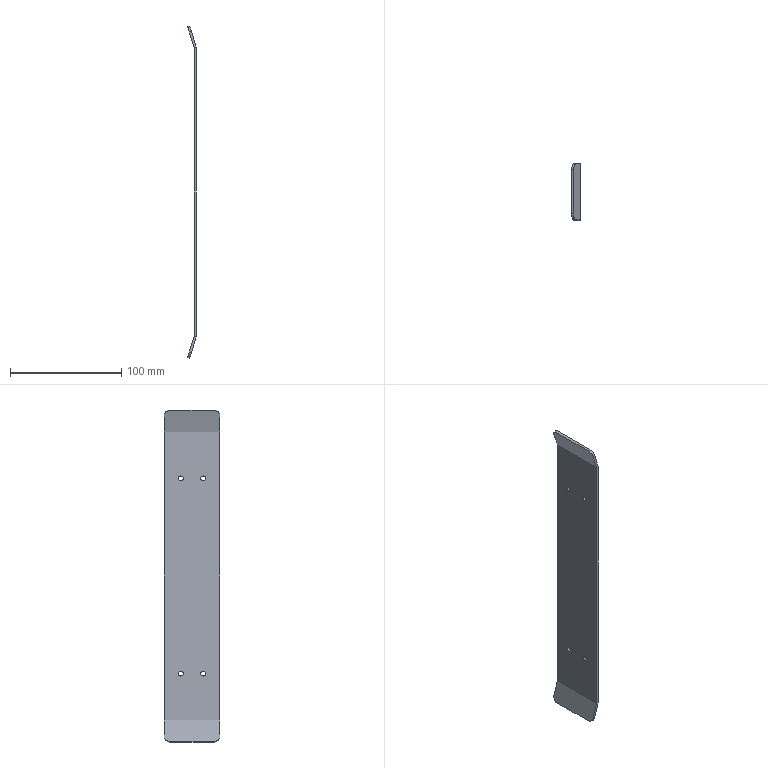Part | SolidWorks | features EdgeFlange 1, Fillet 1, FlatPattern 1, HoleWzd 1, MirrorPattern 1, SMBaseFlange 1, SheetMetal 1 | 1 solid | 34 faces | box 7.789 x 50 x 299.041 mm | volume 29866 mm3 | plane 18 | cylinder 16 | commonest cylinder face diameters 4.2 x10 10 x4 0.2 x2
STEP:
#1=CARTESIAN_POINT('',(-2.,10.,-85.9));
#2=VERTEX_POINT('',#1);
#3=CARTESIAN_POINT('',(-2.,10.,-90.1));
#4=VERTEX_POINT('',#3);
#5=CARTESIAN_POINT('',(-2.,10.,-88.));
#6=DIRECTION('',(1.,0.,0.));
#7=DIRECTION('',(0.,0.,-1.));
#8=AXIS2_PLACEMENT_3D('',#5,#6,#7);
#9=CIRCLE('',#8,2.1);
#10=EDGE_CURVE('',#2,#4,#9,.T.);
#11=ORIENTED_EDGE('',*,*,#10,.F.);
#12=CARTESIAN_POINT('',(0.,10.,-85.9));
#13=VERTEX_POINT('',#12);
#14=CARTESIAN_POINT('',(0.,10.,-85.9));
#15=DIRECTION('',(1.,0.,0.));
#16=VECTOR('',#15,1000.);
#17=LINE('',#14,#16);
#18=EDGE_CURVE('',#2,#13,#17,.T.);
#19=ORIENTED_EDGE('',*,*,#18,.T.);
#20=CARTESIAN_POINT('',(0.,10.,-90.1));
#21=VERTEX_POINT('',#20);
#22=CARTESIAN_POINT('',(0.,10.,-88.));
#23=DIRECTION('',(1.,0.,0.));
#24=DIRECTION('',(0.,0.,-1.));
#25=AXIS2_PLACEMENT_3D('',#22,#23,#24);
#26=CIRCLE('',#25,2.1);
#27=EDGE_CURVE('',#13,#21,#26,.T.);
#28=ORIENTED_EDGE('',*,*,#27,.T.);
#29=CARTESIAN_POINT('',(0.,10.,-90.1));
#30=DIRECTION('',(1.,0.,0.));
#31=VECTOR('',#30,1000.);
#32=LINE('',#29,#31);
#33=EDGE_CURVE('',#4,#21,#32,.T.);
#34=ORIENTED_EDGE('',*,*,#33,.F.);
#35=EDGE_LOOP('',(#11,#19,#28,#34));
#36=FACE_OUTER_BOUND('',#35,.T.);
#37=CARTESIAN_POINT('',(0.,10.,-88.));
#38=DIRECTION('',(1.,0.,0.));
#39=DIRECTION('',(0.,0.,-1.));
#40=AXIS2_PLACEMENT_3D('',#37,#38,#39);
#41=CYLINDRICAL_SURFACE('',#40,2.1);
#42=ADVANCED_FACE('',(#36),#41,.F.);
#43=CARTESIAN_POINT('',(-2.,-10.,-85.9));
#44=VERTEX_POINT('',#43);
#45=CARTESIAN_POINT('',(-2.,-10.,-90.1));
#46=VERTEX_POINT('',#45);
#47=CARTESIAN_POINT('',(-2.,-10.,-88.));
#48=DIRECTION('',(1.,0.,0.));
#49=DIRECTION('',(0.,0.,-1.));
#50=AXIS2_PLACEMENT_3D('',#47,#48,#49);
#51=CIRCLE('',#50,2.1);
#52=EDGE_CURVE('',#44,#46,#51,.T.);
#53=ORIENTED_EDGE('',*,*,#52,.F.);
#54=CARTESIAN_POINT('',(0.,-10.,-85.9));
#55=VERTEX_POINT('',#54);
#56=CARTESIAN_POINT('',(0.,-10.,-85.9));
#57=DIRECTION('',(1.,0.,0.));
#58=VECTOR('',#57,1000.);
#59=LINE('',#56,#58);
#60=EDGE_CURVE('',#44,#55,#59,.T.);
#61=ORIENTED_EDGE('',*,*,#60,.T.);
#62=CARTESIAN_POINT('',(0.,-10.,-90.1));
#63=VERTEX_POINT('',#62);
#64=CARTESIAN_POINT('',(0.,-10.,-88.));
#65=DIRECTION('',(1.,0.,0.));
#66=DIRECTION('',(0.,0.,-1.));
#67=AXIS2_PLACEMENT_3D('',#64,#65,#66);
#68=CIRCLE('',#67,2.1);
#69=EDGE_CURVE('',#55,#63,#68,.T.);
#70=ORIENTED_EDGE('',*,*,#69,.T.);
#71=CARTESIAN_POINT('',(0.,-10.,-90.1));
#72=DIRECTION('',(1.,0.,0.));
#73=VECTOR('',#72,1000.);
#74=LINE('',#71,#73);
#75=EDGE_CURVE('',#46,#63,#74,.T.);
#76=ORIENTED_EDGE('',*,*,#75,.F.);
#77=EDGE_LOOP('',(#53,#61,#70,#76));
#78=FACE_OUTER_BOUND('',#77,.T.);
#79=CARTESIAN_POINT('',(0.,-10.,-88.));
#80=DIRECTION('',(1.,0.,0.));
#81=DIRECTION('',(0.,0.,-1.));
#82=AXIS2_PLACEMENT_3D('',#79,#80,#81);
#83=CYLINDRICAL_SURFACE('',#82,2.1);
#84=ADVANCED_FACE('',(#78),#83,.F.);
#85=CARTESIAN_POINT('',(-2.,10.,90.1));
#86=VERTEX_POINT('',#85);
#87=CARTESIAN_POINT('',(-2.,10.,85.9));
#88=VERTEX_POINT('',#87);
#89=CARTESIAN_POINT('',(-2.,10.,88.));
#90=DIRECTION('',(1.,0.,0.));
#91=DIRECTION('',(0.,0.,-1.));
#92=AXIS2_PLACEMENT_3D('',#89,#90,#91);
#93=CIRCLE('',#92,2.1);
#94=EDGE_CURVE('',#86,#88,#93,.T.);
#95=ORIENTED_EDGE('',*,*,#94,.F.);
#96=CARTESIAN_POINT('',(0.,10.,90.1));
#97=VERTEX_POINT('',#96);
#98=CARTESIAN_POINT('',(0.,10.,90.1));
#99=DIRECTION('',(1.,0.,0.));
#100=VECTOR('',#99,1000.);
#101=LINE('',#98,#100);
#102=EDGE_CURVE('',#86,#97,#101,.T.);
#103=ORIENTED_EDGE('',*,*,#102,.T.);
#104=CARTESIAN_POINT('',(0.,10.,85.9));
#105=VERTEX_POINT('',#104);
#106=CARTESIAN_POINT('',(0.,10.,88.));
#107=DIRECTION('',(1.,0.,0.));
#108=DIRECTION('',(0.,0.,-1.));
#109=AXIS2_PLACEMENT_3D('',#106,#107,#108);
#110=CIRCLE('',#109,2.1);
#111=EDGE_CURVE('',#97,#105,#110,.T.);
#112=ORIENTED_EDGE('',*,*,#111,.T.);
#113=CARTESIAN_POINT('',(0.,10.,85.9));
#114=DIRECTION('',(1.,0.,0.));
#115=VECTOR('',#114,1000.);
#116=LINE('',#113,#115);
#117=EDGE_CURVE('',#88,#105,#116,.T.);
#118=ORIENTED_EDGE('',*,*,#117,.F.);
#119=EDGE_LOOP('',(#95,#103,#112,#118));
#120=FACE_OUTER_BOUND('',#119,.T.);
#121=CARTESIAN_POINT('',(0.,10.,88.));
#122=DIRECTION('',(1.,0.,0.));
#123=DIRECTION('',(0.,0.,-1.));
#124=AXIS2_PLACEMENT_3D('',#121,#122,#123);
#125=CYLINDRICAL_SURFACE('',#124,2.1);
#126=ADVANCED_FACE('',(#120),#125,.F.);
#127=CARTESIAN_POINT('',(-2.,-10.,90.1));
#128=VERTEX_POINT('',#127);
#129=CARTESIAN_POINT('',(-2.,-10.,85.9));
#130=VERTEX_POINT('',#129);
#131=CARTESIAN_POINT('',(-2.,-10.,88.));
#132=DIRECTION('',(1.,0.,0.));
#133=DIRECTION('',(0.,0.,-1.));
#134=AXIS2_PLACEMENT_3D('',#131,#132,#133);
#135=CIRCLE('',#134,2.1);
#136=EDGE_CURVE('',#128,#130,#135,.T.);
#137=ORIENTED_EDGE('',*,*,#136,.F.);
#138=CARTESIAN_POINT('',(0.,-10.,90.1));
#139=VERTEX_POINT('',#138);
#140=CARTESIAN_POINT('',(0.,-10.,90.1));
#141=DIRECTION('',(1.,0.,0.));
#142=VECTOR('',#141,1000.);
#143=LINE('',#140,#142);
#144=EDGE_CURVE('',#128,#139,#143,.T.);
#145=ORIENTED_EDGE('',*,*,#144,.T.);
#146=CARTESIAN_POINT('',(0.,-10.,85.9));
#147=VERTEX_POINT('',#146);
#148=CARTESIAN_POINT('',(0.,-10.,88.));
#149=DIRECTION('',(1.,0.,0.));
#150=DIRECTION('',(0.,0.,-1.));
#151=AXIS2_PLACEMENT_3D('',#148,#149,#150);
#152=CIRCLE('',#151,2.1);
#153=EDGE_CURVE('',#139,#147,#152,.T.);
#154=ORIENTED_EDGE('',*,*,#153,.T.);
#155=CARTESIAN_POINT('',(0.,-10.,85.9));
#156=DIRECTION('',(1.,0.,0.));
#157=VECTOR('',#156,1000.);
#158=LINE('',#155,#157);
#159=EDGE_CURVE('',#130,#147,#158,.T.);
#160=ORIENTED_EDGE('',*,*,#159,.F.);
#161=EDGE_LOOP('',(#137,#145,#154,#160));
#162=FACE_OUTER_BOUND('',#161,.T.);
#163=CARTESIAN_POINT('',(0.,-10.,88.));
#164=DIRECTION('',(1.,0.,0.));
#165=DIRECTION('',(0.,0.,-1.));
#166=AXIS2_PLACEMENT_3D('',#163,#164,#165);
#167=CYLINDRICAL_SURFACE('',#166,2.1);
#168=ADVANCED_FACE('',(#162),#167,.F.);
#169=CARTESIAN_POINT('',(-2.,10.,-88.));
#170=DIRECTION('',(1.,0.,0.));
#171=DIRECTION('',(0.,0.,-1.));
#172=AXIS2_PLACEMENT_3D('',#169,#170,#171);
#173=CIRCLE('',#172,2.1);
#174=EDGE_CURVE('',#4,#2,#173,.T.);
#175=ORIENTED_EDGE('',*,*,#174,.T.);
#176=ORIENTED_EDGE('',*,*,#10,.T.);
#177=EDGE_LOOP('',(#175,#176));
#178=FACE_BOUND('',#177,.T.);
#179=CARTESIAN_POINT('',(-2.,-10.,-88.));
#180=DIRECTION('',(1.,0.,0.));
#181=DIRECTION('',(0.,0.,-1.));
#182=AXIS2_PLACEMENT_3D('',#179,#180,#181);
#183=CIRCLE('',#182,2.1);
#184=EDGE_CURVE('',#46,#44,#183,.T.);
#185=ORIENTED_EDGE('',*,*,#184,.T.);
#186=ORIENTED_EDGE('',*,*,#52,.T.);
#187=EDGE_LOOP('',(#185,#186));
#188=FACE_BOUND('',#187,.T.);
#189=CARTESIAN_POINT('',(-2.,10.,88.));
#190=DIRECTION('',(1.,0.,0.));
#191=DIRECTION('',(0.,0.,-1.));
#192=AXIS2_PLACEMENT_3D('',#189,#190,#191);
#193=CIRCLE('',#192,2.1);
#194=EDGE_CURVE('',#88,#86,#193,.T.);
#195=ORIENTED_EDGE('',*,*,#194,.T.);
#196=ORIENTED_EDGE('',*,*,#94,.T.);
#197=EDGE_LOOP('',(#195,#196));
#198=FACE_BOUND('',#197,.T.);
#199=CARTESIAN_POINT('',(-2.,-10.,88.));
#200=DIRECTION('',(1.,0.,0.));
#201=DIRECTION('',(0.,0.,-1.));
#202=AXIS2_PLACEMENT_3D('',#199,#200,#201);
#203=CIRCLE('',#202,2.1);
#204=EDGE_CURVE('',#130,#128,#203,.T.);
#205=ORIENTED_EDGE('',*,*,#204,.T.);
#206=ORIENTED_EDGE('',*,*,#136,.T.);
#207=EDGE_LOOP('',(#205,#206));
#208=FACE_BOUND('',#207,.T.);
#209=CARTESIAN_POINT('',(-2.,-25.,-129.985));
#210=VERTEX_POINT('',#209);
#211=CARTESIAN_POINT('',(-2.,25.,-129.985));
#212=VERTEX_POINT('',#211);
#213=CARTESIAN_POINT('',(-2.,-25.,-129.985));
#214=DIRECTION('',(0.,1.,0.));
#215=VECTOR('',#214,1000.);
#216=LINE('',#213,#215);
#217=EDGE_CURVE('',#210,#212,#216,.T.);
#218=ORIENTED_EDGE('',*,*,#217,.F.);
#219=CARTESIAN_POINT('',(-2.,-25.,129.985));
#220=VERTEX_POINT('',#219);
#221=CARTESIAN_POINT('',(-2.,-25.,-130.));
#222=DIRECTION('',(0.,0.,-1.));
#223=VECTOR('',#222,1000.);
#224=LINE('',#221,#223);
#225=EDGE_CURVE('',#220,#210,#224,.T.);
#226=ORIENTED_EDGE('',*,*,#225,.F.);
#227=CARTESIAN_POINT('',(-2.,25.,129.985));
#228=VERTEX_POINT('',#227);
#229=CARTESIAN_POINT('',(-2.,25.,129.985));
#230=DIRECTION('',(0.,-1.,0.));
#231=VECTOR('',#230,1000.);
#232=LINE('',#229,#231);
#233=EDGE_CURVE('',#228,#220,#232,.T.);
#234=ORIENTED_EDGE('',*,*,#233,.F.);
#235=CARTESIAN_POINT('',(-2.,25.,-130.));
#236=DIRECTION('',(0.,0.,1.));
#237=VECTOR('',#236,1000.);
#238=LINE('',#235,#237);
#239=EDGE_CURVE('',#212,#228,#238,.T.);
#240=ORIENTED_EDGE('',*,*,#239,.F.);
#241=EDGE_LOOP('',(#218,#226,#234,#240));
#242=FACE_OUTER_BOUND('',#241,.T.);
#243=CARTESIAN_POINT('',(-2.,0.,0.));
#244=DIRECTION('',(1.,0.,0.));
#245=DIRECTION('',(0.,0.,-1.));
#246=AXIS2_PLACEMENT_3D('',#243,#244,#245);
#247=PLANE('',#246);
#248=ADVANCED_FACE('',(#178,#188,#198,#208,#242),#247,.F.);
#249=CARTESIAN_POINT('',(0.,10.,-88.));
#250=DIRECTION('',(1.,0.,0.));
#251=DIRECTION('',(0.,0.,-1.));
#252=AXIS2_PLACEMENT_3D('',#249,#250,#251);
#253=CIRCLE('',#252,2.1);
#254=EDGE_CURVE('',#21,#13,#253,.T.);
#255=ORIENTED_EDGE('',*,*,#254,.F.);
#256=ORIENTED_EDGE('',*,*,#27,.F.);
#257=EDGE_LOOP('',(#255,#256));
#258=FACE_BOUND('',#257,.T.);
#259=CARTESIAN_POINT('',(0.,-10.,-88.));
#260=DIRECTION('',(1.,0.,0.));
#261=DIRECTION('',(0.,0.,-1.));
#262=AXIS2_PLACEMENT_3D('',#259,#260,#261);
#263=CIRCLE('',#262,2.1);
#264=EDGE_CURVE('',#63,#55,#263,.T.);
#265=ORIENTED_EDGE('',*,*,#264,.F.);
#266=ORIENTED_EDGE('',*,*,#69,.F.);
#267=EDGE_LOOP('',(#265,#266));
#268=FACE_BOUND('',#267,.T.);
#269=CARTESIAN_POINT('',(0.,10.,88.));
#270=DIRECTION('',(1.,0.,0.));
#271=DIRECTION('',(0.,0.,-1.));
#272=AXIS2_PLACEMENT_3D('',#269,#270,#271);
#273=CIRCLE('',#272,2.1);
#274=EDGE_CURVE('',#105,#97,#273,.T.);
#275=ORIENTED_EDGE('',*,*,#274,.F.);
#276=ORIENTED_EDGE('',*,*,#111,.F.);
#277=EDGE_LOOP('',(#275,#276));
#278=FACE_BOUND('',#277,.T.);
#279=CARTESIAN_POINT('',(0.,-10.,88.));
#280=DIRECTION('',(1.,0.,0.));
#281=DIRECTION('',(0.,0.,-1.));
#282=AXIS2_PLACEMENT_3D('',#279,#280,#281);
#283=CIRCLE('',#282,2.1);
#284=EDGE_CURVE('',#147,#139,#283,.T.);
#285=ORIENTED_EDGE('',*,*,#284,.F.);
#286=ORIENTED_EDGE('',*,*,#153,.F.);
#287=EDGE_LOOP('',(#285,#286));
#288=FACE_BOUND('',#287,.T.);
#289=CARTESIAN_POINT('',(0.,-25.,129.985));
#290=VERTEX_POINT('',#289);
#291=CARTESIAN_POINT('',(0.,-25.,-129.985));
#292=VERTEX_POINT('',#291);
#293=CARTESIAN_POINT('',(0.,-25.,-130.));
#294=DIRECTION('',(0.,0.,-1.));
#295=VECTOR('',#294,1000.);
#296=LINE('',#293,#295);
#297=EDGE_CURVE('',#290,#292,#296,.T.);
#298=ORIENTED_EDGE('',*,*,#297,.T.);
#299=CARTESIAN_POINT('',(0.,25.,-129.985));
#300=VERTEX_POINT('',#299);
#301=CARTESIAN_POINT('',(0.,-25.,-129.985));
#302=DIRECTION('',(0.,1.,0.));
#303=VECTOR('',#302,1000.);
#304=LINE('',#301,#303);
#305=EDGE_CURVE('',#292,#300,#304,.T.);
#306=ORIENTED_EDGE('',*,*,#305,.T.);
#307=CARTESIAN_POINT('',(0.,25.,129.985));
#308=VERTEX_POINT('',#307);
#309=CARTESIAN_POINT('',(0.,25.,-130.));
#310=DIRECTION('',(0.,0.,1.));
#311=VECTOR('',#310,1000.);
#312=LINE('',#309,#311);
#313=EDGE_CURVE('',#300,#308,#312,.T.);
#314=ORIENTED_EDGE('',*,*,#313,.T.);
#315=CARTESIAN_POINT('',(0.,25.,129.985));
#316=DIRECTION('',(0.,-1.,0.));
#317=VECTOR('',#316,1000.);
#318=LINE('',#315,#317);
#319=EDGE_CURVE('',#308,#290,#318,.T.);
#320=ORIENTED_EDGE('',*,*,#319,.T.);
#321=EDGE_LOOP('',(#298,#306,#314,#320));
#322=FACE_OUTER_BOUND('',#321,.T.);
#323=CARTESIAN_POINT('',(0.,0.,0.));
#324=DIRECTION('',(1.,0.,0.));
#325=DIRECTION('',(0.,0.,-1.));
#326=AXIS2_PLACEMENT_3D('',#323,#324,#325);
#327=PLANE('',#326);
#328=ADVANCED_FACE('',(#258,#268,#278,#288,#322),#327,.T.);
#329=ORIENTED_EDGE('',*,*,#225,.T.);
#330=CARTESIAN_POINT('',(-2.,-25.,-129.985));
#331=DIRECTION('',(1.,0.,0.));
#332=VECTOR('',#331,1000.);
#333=LINE('',#330,#332);
#334=EDGE_CURVE('',#210,#292,#333,.T.);
#335=ORIENTED_EDGE('',*,*,#334,.T.);
#336=ORIENTED_EDGE('',*,*,#297,.F.);
#337=CARTESIAN_POINT('',(-2.,-25.,129.985));
#338=DIRECTION('',(1.,0.,0.));
#339=VECTOR('',#338,1000.);
#340=LINE('',#337,#339);
#341=EDGE_CURVE('',#220,#290,#340,.T.);
#342=ORIENTED_EDGE('',*,*,#341,.F.);
#343=EDGE_LOOP('',(#329,#335,#336,#342));
#344=FACE_OUTER_BOUND('',#343,.T.);
#345=CARTESIAN_POINT('',(-2.,-25.,-130.));
#346=DIRECTION('',(0.,-1.,0.));
#347=DIRECTION('',(0.,0.,-1.));
#348=AXIS2_PLACEMENT_3D('',#345,#346,#347);
#349=PLANE('',#348);
#350=ADVANCED_FACE('',(#344),#349,.T.);
#351=CARTESIAN_POINT('',(-2.,25.,-129.985));
#352=DIRECTION('',(1.,0.,0.));
#353=VECTOR('',#352,1000.);
#354=LINE('',#351,#353);
#355=EDGE_CURVE('',#212,#300,#354,.T.);
#356=ORIENTED_EDGE('',*,*,#355,.F.);
#357=ORIENTED_EDGE('',*,*,#239,.T.);
#358=CARTESIAN_POINT('',(-2.,25.,129.985));
#359=DIRECTION('',(1.,0.,0.));
#360=VECTOR('',#359,1000.);
#361=LINE('',#358,#360);
#362=EDGE_CURVE('',#228,#308,#361,.T.);
#363=ORIENTED_EDGE('',*,*,#362,.T.);
#364=ORIENTED_EDGE('',*,*,#313,.F.);
#365=EDGE_LOOP('',(#356,#357,#363,#364));
#366=FACE_OUTER_BOUND('',#365,.T.);
#367=CARTESIAN_POINT('',(-2.,25.,-130.));
#368=DIRECTION('',(0.,1.,0.));
#369=DIRECTION('',(0.,0.,1.));
#370=AXIS2_PLACEMENT_3D('',#367,#368,#369);
#371=PLANE('',#370);
#372=ADVANCED_FACE('',(#366),#371,.T.);
#373=CARTESIAN_POINT('',(-2.004,-25.,130.014));
#374=VERTEX_POINT('',#373);
#375=CARTESIAN_POINT('',(-0.09176,-25.,130.599));
#376=VERTEX_POINT('',#375);
#377=CARTESIAN_POINT('',(-2.004,-25.,130.014));
#378=DIRECTION('',(0.9563,0.,0.2924));
#379=VECTOR('',#378,1000.);
#380=LINE('',#377,#379);
#381=EDGE_CURVE('',#374,#376,#380,.T.);
#382=ORIENTED_EDGE('',*,*,#381,.F.);
#383=CARTESIAN_POINT('',(-2.1,-25.,129.985));
#384=DIRECTION('',(0.,-1.,0.));
#385=DIRECTION('',(0.,0.,1.));
#386=AXIS2_PLACEMENT_3D('',#383,#384,#385);
#387=CIRCLE('',#386,0.1);
#388=EDGE_CURVE('',#220,#374,#387,.T.);
#389=ORIENTED_EDGE('',*,*,#388,.F.);
#390=ORIENTED_EDGE('',*,*,#341,.T.);
#391=CARTESIAN_POINT('',(-2.1,-25.,129.985));
#392=DIRECTION('',(0.,-1.,0.));
#393=DIRECTION('',(0.,0.,1.));
#394=AXIS2_PLACEMENT_3D('',#391,#392,#393);
#395=CIRCLE('',#394,2.1);
#396=EDGE_CURVE('',#290,#376,#395,.T.);
#397=ORIENTED_EDGE('',*,*,#396,.T.);
#398=EDGE_LOOP('',(#382,#389,#390,#397));
#399=FACE_OUTER_BOUND('',#398,.T.);
#400=CARTESIAN_POINT('',(-2.1,-25.,129.985));
#401=DIRECTION('',(0.,-1.,0.));
#402=DIRECTION('',(0.,0.,-1.));
#403=AXIS2_PLACEMENT_3D('',#400,#401,#402);
#404=PLANE('',#403);
#405=ADVANCED_FACE('',(#399),#404,.T.);
#406=CARTESIAN_POINT('',(-2.004,25.,130.014));
#407=VERTEX_POINT('',#406);
#408=CARTESIAN_POINT('',(-2.1,25.,129.985));
#409=DIRECTION('',(0.,1.,0.));
#410=DIRECTION('',(0.,0.,1.));
#411=AXIS2_PLACEMENT_3D('',#408,#409,#410);
#412=CIRCLE('',#411,0.1);
#413=EDGE_CURVE('',#407,#228,#412,.T.);
#414=ORIENTED_EDGE('',*,*,#413,.F.);
#415=CARTESIAN_POINT('',(-0.09176,25.,130.599));
#416=VERTEX_POINT('',#415);
#417=CARTESIAN_POINT('',(-2.004,25.,130.014));
#418=DIRECTION('',(0.9563,0.,0.2924));
#419=VECTOR('',#418,1000.);
#420=LINE('',#417,#419);
#421=EDGE_CURVE('',#407,#416,#420,.T.);
#422=ORIENTED_EDGE('',*,*,#421,.T.);
#423=CARTESIAN_POINT('',(-2.1,25.,129.985));
#424=DIRECTION('',(0.,1.,0.));
#425=DIRECTION('',(0.,0.,1.));
#426=AXIS2_PLACEMENT_3D('',#423,#424,#425);
#427=CIRCLE('',#426,2.1);
#428=EDGE_CURVE('',#416,#308,#427,.T.);
#429=ORIENTED_EDGE('',*,*,#428,.T.);
#430=ORIENTED_EDGE('',*,*,#362,.F.);
#431=EDGE_LOOP('',(#414,#422,#429,#430));
#432=FACE_OUTER_BOUND('',#431,.T.);
#433=CARTESIAN_POINT('',(-2.1,25.,129.985));
#434=DIRECTION('',(0.,-1.,0.));
#435=DIRECTION('',(0.,0.,-1.));
#436=AXIS2_PLACEMENT_3D('',#433,#434,#435);
#437=PLANE('',#436);
#438=ADVANCED_FACE('',(#432),#437,.F.);
#439=ORIENTED_EDGE('',*,*,#319,.F.);
#440=ORIENTED_EDGE('',*,*,#428,.F.);
#441=CARTESIAN_POINT('',(-0.09176,0.,130.599));
#442=DIRECTION('',(0.,-1.,0.));
#443=VECTOR('',#442,1000.);
#444=LINE('',#441,#443);
#445=EDGE_CURVE('',#416,#376,#444,.T.);
#446=ORIENTED_EDGE('',*,*,#445,.T.);
#447=ORIENTED_EDGE('',*,*,#396,.F.);
#448=EDGE_LOOP('',(#439,#440,#446,#447));
#449=FACE_OUTER_BOUND('',#448,.T.);
#450=CARTESIAN_POINT('',(-2.1,25.,129.985));
#451=DIRECTION('',(0.,1.,0.));
#452=DIRECTION('',(0.9563,0.,0.2924));
#453=AXIS2_PLACEMENT_3D('',#450,#451,#452);
#454=CYLINDRICAL_SURFACE('',#453,2.1);
#455=ADVANCED_FACE('',(#449),#454,.T.);
#456=ORIENTED_EDGE('',*,*,#233,.T.);
#457=ORIENTED_EDGE('',*,*,#388,.T.);
#458=CARTESIAN_POINT('',(-2.004,-25.,130.014));
#459=DIRECTION('',(0.,1.,0.));
#460=VECTOR('',#459,1000.);
#461=LINE('',#458,#460);
#462=EDGE_CURVE('',#374,#407,#461,.T.);
#463=ORIENTED_EDGE('',*,*,#462,.T.);
#464=ORIENTED_EDGE('',*,*,#413,.T.);
#465=EDGE_LOOP('',(#456,#457,#463,#464));
#466=FACE_OUTER_BOUND('',#465,.T.);
#467=CARTESIAN_POINT('',(-2.1,25.,129.985));
#468=DIRECTION('',(0.,1.,0.));
#469=DIRECTION('',(0.9563,0.,0.2924));
#470=AXIS2_PLACEMENT_3D('',#467,#468,#469);
#471=CYLINDRICAL_SURFACE('',#470,0.1);
#472=ADVANCED_FACE('',(#466),#471,.F.);
#473=CARTESIAN_POINT('',(-6.327,25.,144.154));
#474=VERTEX_POINT('',#473);
#475=CARTESIAN_POINT('',(-7.789,25.,148.936));
#476=DIRECTION('',(-0.2924,0.,0.9563));
#477=VECTOR('',#476,1000.);
#478=LINE('',#475,#477);
#479=EDGE_CURVE('',#407,#474,#478,.T.);
#480=ORIENTED_EDGE('',*,*,#479,.T.);
#481=CARTESIAN_POINT('',(-4.415,25.,144.739));
#482=VERTEX_POINT('',#481);
#483=CARTESIAN_POINT('',(-4.415,25.,144.739));
#484=DIRECTION('',(0.9563,0.,0.2924));
#485=VECTOR('',#484,1000.);
#486=LINE('',#483,#485);
#487=EDGE_CURVE('',#474,#482,#486,.T.);
#488=ORIENTED_EDGE('',*,*,#487,.T.);
#489=CARTESIAN_POINT('',(-5.877,25.,149.521));
#490=DIRECTION('',(-0.2924,0.,0.9563));
#491=VECTOR('',#490,1000.);
#492=LINE('',#489,#491);
#493=EDGE_CURVE('',#416,#482,#492,.T.);
#494=ORIENTED_EDGE('',*,*,#493,.F.);
#495=ORIENTED_EDGE('',*,*,#421,.F.);
#496=EDGE_LOOP('',(#480,#488,#494,#495));
#497=FACE_OUTER_BOUND('',#496,.T.);
#498=CARTESIAN_POINT('',(-5.877,25.,149.521));
#499=DIRECTION('',(0.,-1.,0.));
#500=DIRECTION('',(0.,0.,-1.));
#501=AXIS2_PLACEMENT_3D('',#498,#499,#500);
#502=PLANE('',#501);
#503=ADVANCED_FACE('',(#497),#502,.F.);
#504=CARTESIAN_POINT('',(-4.415,-25.,144.739));
#505=VERTEX_POINT('',#504);
#506=CARTESIAN_POINT('',(-0.08739,-25.,130.585));
#507=DIRECTION('',(0.2924,0.,-0.9563));
#508=VECTOR('',#507,1000.);
#509=LINE('',#506,#508);
#510=EDGE_CURVE('',#505,#376,#509,.T.);
#511=ORIENTED_EDGE('',*,*,#510,.F.);
#512=CARTESIAN_POINT('',(-6.327,-25.,144.154));
#513=VERTEX_POINT('',#512);
#514=CARTESIAN_POINT('',(-4.415,-25.,144.739));
#515=DIRECTION('',(-0.9563,0.,-0.2924));
#516=VECTOR('',#515,1000.);
#517=LINE('',#514,#516);
#518=EDGE_CURVE('',#505,#513,#517,.T.);
#519=ORIENTED_EDGE('',*,*,#518,.T.);
#520=CARTESIAN_POINT('',(-2.,-25.,130.));
#521=DIRECTION('',(0.2924,0.,-0.9563));
#522=VECTOR('',#521,1000.);
#523=LINE('',#520,#522);
#524=EDGE_CURVE('',#513,#374,#523,.T.);
#525=ORIENTED_EDGE('',*,*,#524,.T.);
#526=ORIENTED_EDGE('',*,*,#381,.T.);
#527=EDGE_LOOP('',(#511,#519,#525,#526));
#528=FACE_OUTER_BOUND('',#527,.T.);
#529=CARTESIAN_POINT('',(-0.08739,-25.,130.585));
#530=DIRECTION('',(0.,1.,0.));
#531=DIRECTION('',(0.,0.,1.));
#532=AXIS2_PLACEMENT_3D('',#529,#530,#531);
#533=PLANE('',#532);
#534=ADVANCED_FACE('',(#528),#533,.F.);
#535=CARTESIAN_POINT('',(-5.877,20.,149.521));
#536=VERTEX_POINT('',#535);
#537=CARTESIAN_POINT('',(-5.877,-20.,149.521));
#538=VERTEX_POINT('',#537);
#539=CARTESIAN_POINT('',(-5.877,-25.,149.521));
#540=DIRECTION('',(0.,-1.,0.));
#541=VECTOR('',#540,1000.);
#542=LINE('',#539,#541);
#543=EDGE_CURVE('',#536,#538,#542,.T.);
#544=ORIENTED_EDGE('',*,*,#543,.T.);
#545=CARTESIAN_POINT('',(-4.415,-20.,144.739));
#546=DIRECTION('',(0.9563,0.,0.2924));
#547=DIRECTION('',(-0.2924,0.,0.9563));
#548=AXIS2_PLACEMENT_3D('',#545,#546,#547);
#549=CIRCLE('',#548,5.);
#550=EDGE_CURVE('',#538,#505,#549,.T.);
#551=ORIENTED_EDGE('',*,*,#550,.T.);
#552=ORIENTED_EDGE('',*,*,#510,.T.);
#553=ORIENTED_EDGE('',*,*,#445,.F.);
#554=ORIENTED_EDGE('',*,*,#493,.T.);
#555=CARTESIAN_POINT('',(-4.415,20.,144.739));
#556=DIRECTION('',(0.9563,0.,0.2924));
#557=DIRECTION('',(-0.2924,0.,0.9563));
#558=AXIS2_PLACEMENT_3D('',#555,#556,#557);
#559=CIRCLE('',#558,5.);
#560=EDGE_CURVE('',#482,#536,#559,.T.);
#561=ORIENTED_EDGE('',*,*,#560,.T.);
#562=EDGE_LOOP('',(#544,#551,#552,#553,#554,#561));
#563=FACE_OUTER_BOUND('',#562,.T.);
#564=CARTESIAN_POINT('',(36.431,0.,11.138));
#565=DIRECTION('',(-0.9563,0.,-0.2924));
#566=DIRECTION('',(-0.2924,0.,0.9563));
#567=AXIS2_PLACEMENT_3D('',#564,#565,#566);
#568=PLANE('',#567);
#569=ADVANCED_FACE('',(#563),#568,.F.);
#570=ORIENTED_EDGE('',*,*,#524,.F.);
#571=CARTESIAN_POINT('',(-7.789,-20.,148.936));
#572=VERTEX_POINT('',#571);
#573=CARTESIAN_POINT('',(-6.327,-20.,144.154));
#574=DIRECTION('',(-0.9563,0.,-0.2924));
#575=DIRECTION('',(-0.2924,0.,0.9563));
#576=AXIS2_PLACEMENT_3D('',#573,#574,#575);
#577=CIRCLE('',#576,5.);
#578=EDGE_CURVE('',#513,#572,#577,.T.);
#579=ORIENTED_EDGE('',*,*,#578,.T.);
#580=CARTESIAN_POINT('',(-7.789,20.,148.936));
#581=VERTEX_POINT('',#580);
#582=CARTESIAN_POINT('',(-7.789,-25.,148.936));
#583=DIRECTION('',(0.,-1.,0.));
#584=VECTOR('',#583,1000.);
#585=LINE('',#582,#584);
#586=EDGE_CURVE('',#581,#572,#585,.T.);
#587=ORIENTED_EDGE('',*,*,#586,.F.);
#588=CARTESIAN_POINT('',(-6.327,20.,144.154));
#589=DIRECTION('',(-0.9563,0.,-0.2924));
#590=DIRECTION('',(-0.2924,0.,0.9563));
#591=AXIS2_PLACEMENT_3D('',#588,#589,#590);
#592=CIRCLE('',#591,5.);
#593=EDGE_CURVE('',#581,#474,#592,.T.);
#594=ORIENTED_EDGE('',*,*,#593,.T.);
#595=ORIENTED_EDGE('',*,*,#479,.F.);
#596=ORIENTED_EDGE('',*,*,#462,.F.);
#597=EDGE_LOOP('',(#570,#579,#587,#594,#595,#596));
#598=FACE_OUTER_BOUND('',#597,.T.);
#599=CARTESIAN_POINT('',(34.519,0.,10.553));
#600=DIRECTION('',(-0.9563,0.,-0.2924));
#601=DIRECTION('',(-0.2924,0.,0.9563));
#602=AXIS2_PLACEMENT_3D('',#599,#600,#601);
#603=PLANE('',#602);
#604=ADVANCED_FACE('',(#598),#603,.T.);
#605=ORIENTED_EDGE('',*,*,#586,.T.);
#606=CARTESIAN_POINT('',(-5.877,-20.,149.521));
#607=DIRECTION('',(0.9563,0.,0.2924));
#608=VECTOR('',#607,1000.);
#609=LINE('',#606,#608);
#610=EDGE_CURVE('',#572,#538,#609,.T.);
#611=ORIENTED_EDGE('',*,*,#610,.T.);
#612=ORIENTED_EDGE('',*,*,#543,.F.);
#613=CARTESIAN_POINT('',(-5.877,20.,149.521));
#614=DIRECTION('',(-0.9563,0.,-0.2924));
#615=VECTOR('',#614,1000.);
#616=LINE('',#613,#615);
#617=EDGE_CURVE('',#536,#581,#616,.T.);
#618=ORIENTED_EDGE('',*,*,#617,.T.);
#619=EDGE_LOOP('',(#605,#611,#612,#618));
#620=FACE_OUTER_BOUND('',#619,.T.);
#621=CARTESIAN_POINT('',(-5.877,-25.,149.521));
#622=DIRECTION('',(0.2924,0.,-0.9563));
#623=DIRECTION('',(-0.9563,0.,-0.2924));
#624=AXIS2_PLACEMENT_3D('',#621,#622,#623);
#625=PLANE('',#624);
#626=ADVANCED_FACE('',(#620),#625,.F.);
#627=CARTESIAN_POINT('',(-2.004,25.,-130.014));
#628=VERTEX_POINT('',#627);
#629=CARTESIAN_POINT('',(-0.09176,25.,-130.599));
#630=VERTEX_POINT('',#629);
#631=CARTESIAN_POINT('',(-2.004,25.,-130.014));
#632=DIRECTION('',(0.9563,0.,-0.2924));
#633=VECTOR('',#632,1000.);
#634=LINE('',#631,#633);
#635=EDGE_CURVE('',#628,#630,#634,.T.);
#636=ORIENTED_EDGE('',*,*,#635,.F.);
#637=CARTESIAN_POINT('',(-2.1,25.,-129.985));
#638=DIRECTION('',(0.,1.,0.));
#639=DIRECTION('',(0.,0.,-1.));
#640=AXIS2_PLACEMENT_3D('',#637,#638,#639);
#641=CIRCLE('',#640,0.1);
#642=EDGE_CURVE('',#212,#628,#641,.T.);
#643=ORIENTED_EDGE('',*,*,#642,.F.);
#644=ORIENTED_EDGE('',*,*,#355,.T.);
#645=CARTESIAN_POINT('',(-2.1,25.,-129.985));
#646=DIRECTION('',(0.,1.,0.));
#647=DIRECTION('',(0.,0.,-1.));
#648=AXIS2_PLACEMENT_3D('',#645,#646,#647);
#649=CIRCLE('',#648,2.1);
#650=EDGE_CURVE('',#300,#630,#649,.T.);
#651=ORIENTED_EDGE('',*,*,#650,.T.);
#652=EDGE_LOOP('',(#636,#643,#644,#651));
#653=FACE_OUTER_BOUND('',#652,.T.);
#654=CARTESIAN_POINT('',(-2.1,25.,-129.985));
#655=DIRECTION('',(0.,1.,0.));
#656=DIRECTION('',(0.,0.,1.));
#657=AXIS2_PLACEMENT_3D('',#654,#655,#656);
#658=PLANE('',#657);
#659=ADVANCED_FACE('',(#653),#658,.T.);
#660=CARTESIAN_POINT('',(-2.004,-25.,-130.014));
#661=VERTEX_POINT('',#660);
#662=CARTESIAN_POINT('',(-2.1,-25.,-129.985));
#663=DIRECTION('',(0.,-1.,0.));
#664=DIRECTION('',(0.,0.,-1.));
#665=AXIS2_PLACEMENT_3D('',#662,#663,#664);
#666=CIRCLE('',#665,0.1);
#667=EDGE_CURVE('',#661,#210,#666,.T.);
#668=ORIENTED_EDGE('',*,*,#667,.F.);
#669=CARTESIAN_POINT('',(-0.09176,-25.,-130.599));
#670=VERTEX_POINT('',#669);
#671=CARTESIAN_POINT('',(-2.004,-25.,-130.014));
#672=DIRECTION('',(0.9563,0.,-0.2924));
#673=VECTOR('',#672,1000.);
#674=LINE('',#671,#673);
#675=EDGE_CURVE('',#661,#670,#674,.T.);
#676=ORIENTED_EDGE('',*,*,#675,.T.);
#677=CARTESIAN_POINT('',(-2.1,-25.,-129.985));
#678=DIRECTION('',(0.,-1.,0.));
#679=DIRECTION('',(0.,0.,-1.));
#680=AXIS2_PLACEMENT_3D('',#677,#678,#679);
#681=CIRCLE('',#680,2.1);
#682=EDGE_CURVE('',#670,#292,#681,.T.);
#683=ORIENTED_EDGE('',*,*,#682,.T.);
#684=ORIENTED_EDGE('',*,*,#334,.F.);
#685=EDGE_LOOP('',(#668,#676,#683,#684));
#686=FACE_OUTER_BOUND('',#685,.T.);
#687=CARTESIAN_POINT('',(-2.1,-25.,-129.985));
#688=DIRECTION('',(0.,1.,0.));
#689=DIRECTION('',(0.,0.,1.));
#690=AXIS2_PLACEMENT_3D('',#687,#688,#689);
#691=PLANE('',#690);
#692=ADVANCED_FACE('',(#686),#691,.F.);
#693=ORIENTED_EDGE('',*,*,#305,.F.);
#694=ORIENTED_EDGE('',*,*,#682,.F.);
#695=CARTESIAN_POINT('',(-0.09176,0.,-130.599));
#696=DIRECTION('',(0.,1.,0.));
#697=VECTOR('',#696,1000.);
#698=LINE('',#695,#697);
#699=EDGE_CURVE('',#670,#630,#698,.T.);
#700=ORIENTED_EDGE('',*,*,#699,.T.);
#701=ORIENTED_EDGE('',*,*,#650,.F.);
#702=EDGE_LOOP('',(#693,#694,#700,#701));
#703=FACE_OUTER_BOUND('',#702,.T.);
#704=CARTESIAN_POINT('',(-2.1,-25.,-129.985));
#705=DIRECTION('',(0.,-1.,0.));
#706=DIRECTION('',(0.9563,0.,-0.2924));
#707=AXIS2_PLACEMENT_3D('',#704,#705,#706);
#708=CYLINDRICAL_SURFACE('',#707,2.1);
#709=ADVANCED_FACE('',(#703),#708,.T.);
#710=ORIENTED_EDGE('',*,*,#217,.T.);
#711=ORIENTED_EDGE('',*,*,#642,.T.);
#712=CARTESIAN_POINT('',(-2.004,25.,-130.014));
#713=DIRECTION('',(0.,-1.,0.));
#714=VECTOR('',#713,1000.);
#715=LINE('',#712,#714);
#716=EDGE_CURVE('',#628,#661,#715,.T.);
#717=ORIENTED_EDGE('',*,*,#716,.T.);
#718=ORIENTED_EDGE('',*,*,#667,.T.);
#719=EDGE_LOOP('',(#710,#711,#717,#718));
#720=FACE_OUTER_BOUND('',#719,.T.);
#721=CARTESIAN_POINT('',(-2.1,-25.,-129.985));
#722=DIRECTION('',(0.,-1.,0.));
#723=DIRECTION('',(0.9563,0.,-0.2924));
#724=AXIS2_PLACEMENT_3D('',#721,#722,#723);
#725=CYLINDRICAL_SURFACE('',#724,0.1);
#726=ADVANCED_FACE('',(#720),#725,.F.);
#727=CARTESIAN_POINT('',(-6.327,-25.,-144.154));
#728=VERTEX_POINT('',#727);
#729=CARTESIAN_POINT('',(-7.789,-25.,-148.936));
#730=DIRECTION('',(-0.2924,0.,-0.9563));
#731=VECTOR('',#730,1000.);
#732=LINE('',#729,#731);
#733=EDGE_CURVE('',#661,#728,#732,.T.);
#734=ORIENTED_EDGE('',*,*,#733,.T.);
#735=CARTESIAN_POINT('',(-4.415,-25.,-144.739));
#736=VERTEX_POINT('',#735);
#737=CARTESIAN_POINT('',(-4.415,-25.,-144.739));
#738=DIRECTION('',(0.9563,0.,-0.2924));
#739=VECTOR('',#738,1000.);
#740=LINE('',#737,#739);
#741=EDGE_CURVE('',#728,#736,#740,.T.);
#742=ORIENTED_EDGE('',*,*,#741,.T.);
#743=CARTESIAN_POINT('',(-5.877,-25.,-149.521));
#744=DIRECTION('',(-0.2924,0.,-0.9563));
#745=VECTOR('',#744,1000.);
#746=LINE('',#743,#745);
#747=EDGE_CURVE('',#670,#736,#746,.T.);
#748=ORIENTED_EDGE('',*,*,#747,.F.);
#749=ORIENTED_EDGE('',*,*,#675,.F.);
#750=EDGE_LOOP('',(#734,#742,#748,#749));
#751=FACE_OUTER_BOUND('',#750,.T.);
#752=CARTESIAN_POINT('',(-5.877,-25.,-149.521));
#753=DIRECTION('',(0.,1.,0.));
#754=DIRECTION('',(0.,0.,1.));
#755=AXIS2_PLACEMENT_3D('',#752,#753,#754);
#756=PLANE('',#755);
#757=ADVANCED_FACE('',(#751),#756,.F.);
#758=CARTESIAN_POINT('',(-4.415,25.,-144.739));
#759=VERTEX_POINT('',#758);
#760=CARTESIAN_POINT('',(-0.08739,25.,-130.585));
#761=DIRECTION('',(0.2924,0.,0.9563));
#762=VECTOR('',#761,1000.);
#763=LINE('',#760,#762);
#764=EDGE_CURVE('',#759,#630,#763,.T.);
#765=ORIENTED_EDGE('',*,*,#764,.F.);
#766=CARTESIAN_POINT('',(-6.327,25.,-144.154));
#767=VERTEX_POINT('',#766);
#768=CARTESIAN_POINT('',(-4.415,25.,-144.739));
#769=DIRECTION('',(-0.9563,0.,0.2924));
#770=VECTOR('',#769,1000.);
#771=LINE('',#768,#770);
#772=EDGE_CURVE('',#759,#767,#771,.T.);
#773=ORIENTED_EDGE('',*,*,#772,.T.);
#774=CARTESIAN_POINT('',(-2.,25.,-130.));
#775=DIRECTION('',(0.2924,0.,0.9563));
#776=VECTOR('',#775,1000.);
#777=LINE('',#774,#776);
#778=EDGE_CURVE('',#767,#628,#777,.T.);
#779=ORIENTED_EDGE('',*,*,#778,.T.);
#780=ORIENTED_EDGE('',*,*,#635,.T.);
#781=EDGE_LOOP('',(#765,#773,#779,#780));
#782=FACE_OUTER_BOUND('',#781,.T.);
#783=CARTESIAN_POINT('',(-0.08739,25.,-130.585));
#784=DIRECTION('',(0.,-1.,0.));
#785=DIRECTION('',(0.,0.,-1.));
#786=AXIS2_PLACEMENT_3D('',#783,#784,#785);
#787=PLANE('',#786);
#788=ADVANCED_FACE('',(#782),#787,.F.);
#789=ORIENTED_EDGE('',*,*,#747,.T.);
#790=CARTESIAN_POINT('',(-5.877,-20.,-149.521));
#791=VERTEX_POINT('',#790);
#792=CARTESIAN_POINT('',(-4.415,-20.,-144.739));
#793=DIRECTION('',(0.9563,0.,-0.2924));
#794=DIRECTION('',(0.2924,0.,0.9563));
#795=AXIS2_PLACEMENT_3D('',#792,#793,#794);
#796=CIRCLE('',#795,5.);
#797=EDGE_CURVE('',#736,#791,#796,.T.);
#798=ORIENTED_EDGE('',*,*,#797,.T.);
#799=CARTESIAN_POINT('',(-5.877,20.,-149.521));
#800=VERTEX_POINT('',#799);
#801=CARTESIAN_POINT('',(-5.877,25.,-149.521));
#802=DIRECTION('',(0.,1.,0.));
#803=VECTOR('',#802,1000.);
#804=LINE('',#801,#803);
#805=EDGE_CURVE('',#791,#800,#804,.T.);
#806=ORIENTED_EDGE('',*,*,#805,.T.);
#807=CARTESIAN_POINT('',(-4.415,20.,-144.739));
#808=DIRECTION('',(0.9563,0.,-0.2924));
#809=DIRECTION('',(0.2924,0.,0.9563));
#810=AXIS2_PLACEMENT_3D('',#807,#808,#809);
#811=CIRCLE('',#810,5.);
#812=EDGE_CURVE('',#800,#759,#811,.T.);
#813=ORIENTED_EDGE('',*,*,#812,.T.);
#814=ORIENTED_EDGE('',*,*,#764,.T.);
#815=ORIENTED_EDGE('',*,*,#699,.F.);
#816=EDGE_LOOP('',(#789,#798,#806,#813,#814,#815));
#817=FACE_OUTER_BOUND('',#816,.T.);
#818=CARTESIAN_POINT('',(36.431,0.,-11.138));
#819=DIRECTION('',(-0.9563,0.,0.2924));
#820=DIRECTION('',(0.2924,0.,0.9563));
#821=AXIS2_PLACEMENT_3D('',#818,#819,#820);
#822=PLANE('',#821);
#823=ADVANCED_FACE('',(#817),#822,.F.);
#824=CARTESIAN_POINT('',(-7.789,-20.,-148.936));
#825=VERTEX_POINT('',#824);
#826=CARTESIAN_POINT('',(-7.789,20.,-148.936));
#827=VERTEX_POINT('',#826);
#828=CARTESIAN_POINT('',(-7.789,25.,-148.936));
#829=DIRECTION('',(0.,1.,0.));
#830=VECTOR('',#829,1000.);
#831=LINE('',#828,#830);
#832=EDGE_CURVE('',#825,#827,#831,.T.);
#833=ORIENTED_EDGE('',*,*,#832,.F.);
#834=CARTESIAN_POINT('',(-6.327,-20.,-144.154));
#835=DIRECTION('',(-0.9563,0.,0.2924));
#836=DIRECTION('',(0.2924,0.,0.9563));
#837=AXIS2_PLACEMENT_3D('',#834,#835,#836);
#838=CIRCLE('',#837,5.);
#839=EDGE_CURVE('',#825,#728,#838,.T.);
#840=ORIENTED_EDGE('',*,*,#839,.T.);
#841=ORIENTED_EDGE('',*,*,#733,.F.);
#842=ORIENTED_EDGE('',*,*,#716,.F.);
#843=ORIENTED_EDGE('',*,*,#778,.F.);
#844=CARTESIAN_POINT('',(-6.327,20.,-144.154));
#845=DIRECTION('',(-0.9563,0.,0.2924));
#846=DIRECTION('',(0.2924,0.,0.9563));
#847=AXIS2_PLACEMENT_3D('',#844,#845,#846);
#848=CIRCLE('',#847,5.);
#849=EDGE_CURVE('',#767,#827,#848,.T.);
#850=ORIENTED_EDGE('',*,*,#849,.T.);
#851=EDGE_LOOP('',(#833,#840,#841,#842,#843,#850));
#852=FACE_OUTER_BOUND('',#851,.T.);
#853=CARTESIAN_POINT('',(34.519,0.,-10.553));
#854=DIRECTION('',(-0.9563,0.,0.2924));
#855=DIRECTION('',(0.2924,0.,0.9563));
#856=AXIS2_PLACEMENT_3D('',#853,#854,#855);
#857=PLANE('',#856);
#858=ADVANCED_FACE('',(#852),#857,.T.);
#859=ORIENTED_EDGE('',*,*,#805,.F.);
#860=CARTESIAN_POINT('',(-5.877,-20.,-149.521));
#861=DIRECTION('',(-0.9563,0.,0.2924));
#862=VECTOR('',#861,1000.);
#863=LINE('',#860,#862);
#864=EDGE_CURVE('',#791,#825,#863,.T.);
#865=ORIENTED_EDGE('',*,*,#864,.T.);
#866=ORIENTED_EDGE('',*,*,#832,.T.);
#867=CARTESIAN_POINT('',(-5.877,20.,-149.521));
#868=DIRECTION('',(0.9563,0.,-0.2924));
#869=VECTOR('',#868,1000.);
#870=LINE('',#867,#869);
#871=EDGE_CURVE('',#827,#800,#870,.T.);
#872=ORIENTED_EDGE('',*,*,#871,.T.);
#873=EDGE_LOOP('',(#859,#865,#866,#872));
#874=FACE_OUTER_BOUND('',#873,.T.);
#875=CARTESIAN_POINT('',(-5.877,25.,-149.521));
#876=DIRECTION('',(0.2924,0.,0.9563));
#877=DIRECTION('',(0.9563,0.,-0.2924));
#878=AXIS2_PLACEMENT_3D('',#875,#876,#877);
#879=PLANE('',#878);
#880=ADVANCED_FACE('',(#874),#879,.F.);
#881=ORIENTED_EDGE('',*,*,#144,.F.);
#882=ORIENTED_EDGE('',*,*,#204,.F.);
#883=ORIENTED_EDGE('',*,*,#159,.T.);
#884=ORIENTED_EDGE('',*,*,#284,.T.);
#885=EDGE_LOOP('',(#881,#882,#883,#884));
#886=FACE_OUTER_BOUND('',#885,.T.);
#887=CARTESIAN_POINT('',(0.,-10.,88.));
#888=DIRECTION('',(1.,0.,0.));
#889=DIRECTION('',(0.,0.,-1.));
#890=AXIS2_PLACEMENT_3D('',#887,#888,#889);
#891=CYLINDRICAL_SURFACE('',#890,2.1);
#892=ADVANCED_FACE('',(#886),#891,.F.);
#893=ORIENTED_EDGE('',*,*,#102,.F.);
#894=ORIENTED_EDGE('',*,*,#194,.F.);
#895=ORIENTED_EDGE('',*,*,#117,.T.);
#896=ORIENTED_EDGE('',*,*,#274,.T.);
#897=EDGE_LOOP('',(#893,#894,#895,#896));
#898=FACE_OUTER_BOUND('',#897,.T.);
#899=CARTESIAN_POINT('',(0.,10.,88.));
#900=DIRECTION('',(1.,0.,0.));
#901=DIRECTION('',(0.,0.,-1.));
#902=AXIS2_PLACEMENT_3D('',#899,#900,#901);
#903=CYLINDRICAL_SURFACE('',#902,2.1);
#904=ADVANCED_FACE('',(#898),#903,.F.);
#905=ORIENTED_EDGE('',*,*,#60,.F.);
#906=ORIENTED_EDGE('',*,*,#184,.F.);
#907=ORIENTED_EDGE('',*,*,#75,.T.);
#908=ORIENTED_EDGE('',*,*,#264,.T.);
#909=EDGE_LOOP('',(#905,#906,#907,#908));
#910=FACE_OUTER_BOUND('',#909,.T.);
#911=CARTESIAN_POINT('',(0.,-10.,-88.));
#912=DIRECTION('',(1.,0.,0.));
#913=DIRECTION('',(0.,0.,-1.));
#914=AXIS2_PLACEMENT_3D('',#911,#912,#913);
#915=CYLINDRICAL_SURFACE('',#914,2.1);
#916=ADVANCED_FACE('',(#910),#915,.F.);
#917=ORIENTED_EDGE('',*,*,#18,.F.);
#918=ORIENTED_EDGE('',*,*,#174,.F.);
#919=ORIENTED_EDGE('',*,*,#33,.T.);
#920=ORIENTED_EDGE('',*,*,#254,.T.);
#921=EDGE_LOOP('',(#917,#918,#919,#920));
#922=FACE_OUTER_BOUND('',#921,.T.);
#923=CARTESIAN_POINT('',(0.,10.,-88.));
#924=DIRECTION('',(1.,0.,0.));
#925=DIRECTION('',(0.,0.,-1.));
#926=AXIS2_PLACEMENT_3D('',#923,#924,#925);
#927=CYLINDRICAL_SURFACE('',#926,2.1);
#928=ADVANCED_FACE('',(#922),#927,.F.);
#929=ORIENTED_EDGE('',*,*,#797,.F.);
#930=ORIENTED_EDGE('',*,*,#741,.F.);
#931=ORIENTED_EDGE('',*,*,#839,.F.);
#932=ORIENTED_EDGE('',*,*,#864,.F.);
#933=EDGE_LOOP('',(#929,#930,#931,#932));
#934=FACE_OUTER_BOUND('',#933,.T.);
#935=CARTESIAN_POINT('',(-4.415,-20.,-144.739));
#936=DIRECTION('',(-0.9563,0.,0.2924));
#937=DIRECTION('',(0.2924,0.,0.9563));
#938=AXIS2_PLACEMENT_3D('',#935,#936,#937);
#939=CYLINDRICAL_SURFACE('',#938,5.);
#940=ADVANCED_FACE('',(#934),#939,.T.);
#941=ORIENTED_EDGE('',*,*,#812,.F.);
#942=ORIENTED_EDGE('',*,*,#871,.F.);
#943=ORIENTED_EDGE('',*,*,#849,.F.);
#944=ORIENTED_EDGE('',*,*,#772,.F.);
#945=EDGE_LOOP('',(#941,#942,#943,#944));
#946=FACE_OUTER_BOUND('',#945,.T.);
#947=CARTESIAN_POINT('',(-4.415,20.,-144.739));
#948=DIRECTION('',(-0.9563,0.,0.2924));
#949=DIRECTION('',(0.2924,0.,0.9563));
#950=AXIS2_PLACEMENT_3D('',#947,#948,#949);
#951=CYLINDRICAL_SURFACE('',#950,5.);
#952=ADVANCED_FACE('',(#946),#951,.T.);
#953=ORIENTED_EDGE('',*,*,#550,.F.);
#954=ORIENTED_EDGE('',*,*,#610,.F.);
#955=ORIENTED_EDGE('',*,*,#578,.F.);
#956=ORIENTED_EDGE('',*,*,#518,.F.);
#957=EDGE_LOOP('',(#953,#954,#955,#956));
#958=FACE_OUTER_BOUND('',#957,.T.);
#959=CARTESIAN_POINT('',(-4.415,-20.,144.739));
#960=DIRECTION('',(-0.9563,0.,-0.2924));
#961=DIRECTION('',(-0.2924,0.,0.9563));
#962=AXIS2_PLACEMENT_3D('',#959,#960,#961);
#963=CYLINDRICAL_SURFACE('',#962,5.);
#964=ADVANCED_FACE('',(#958),#963,.T.);
#965=ORIENTED_EDGE('',*,*,#560,.F.);
#966=ORIENTED_EDGE('',*,*,#487,.F.);
#967=ORIENTED_EDGE('',*,*,#593,.F.);
#968=ORIENTED_EDGE('',*,*,#617,.F.);
#969=EDGE_LOOP('',(#965,#966,#967,#968));
#970=FACE_OUTER_BOUND('',#969,.T.);
#971=CARTESIAN_POINT('',(-4.415,20.,144.739));
#972=DIRECTION('',(-0.9563,0.,-0.2924));
#973=DIRECTION('',(-0.2924,0.,0.9563));
#974=AXIS2_PLACEMENT_3D('',#971,#972,#973);
#975=CYLINDRICAL_SURFACE('',#974,5.);
#976=ADVANCED_FACE('',(#970),#975,.T.);
#977=CLOSED_SHELL('',(#42,#84,#126,#168,#248,#328,#350,#372,#405,#438,#455,#472,#503,#534,#569,#604,#626,#659,#692,#709,#726,#757,#788,#823,#858,#880,#892,#904,#916,#928,#940,#952,#964,#976));
#978=MANIFOLD_SOLID_BREP('',#977);
#979=CARTESIAN_POINT('',(0.,0.,0.));
#980=DIRECTION('',(0.,0.,1.));
#981=DIRECTION('',(1.,0.,0.));
#982=AXIS2_PLACEMENT_3D('',#979,#980,#981);
#983=(LENGTH_UNIT()NAMED_UNIT(*)SI_UNIT(.MILLI.,.METRE.));
#984=UNCERTAINTY_MEASURE_WITH_UNIT(LENGTH_MEASURE(0.00001),#983,'','');
#985=(NAMED_UNIT(*)PLANE_ANGLE_UNIT()SI_UNIT($,.RADIAN.));
#986=(NAMED_UNIT(*)SI_UNIT($,.STERADIAN.)SOLID_ANGLE_UNIT());
#987=(GEOMETRIC_REPRESENTATION_CONTEXT(3)GLOBAL_UNCERTAINTY_ASSIGNED_CONTEXT((#984))GLOBAL_UNIT_ASSIGNED_CONTEXT((#983,#985,#986))REPRESENTATION_CONTEXT('',''));
#988=ADVANCED_BREP_SHAPE_REPRESENTATION('',(#978,#982),#987);